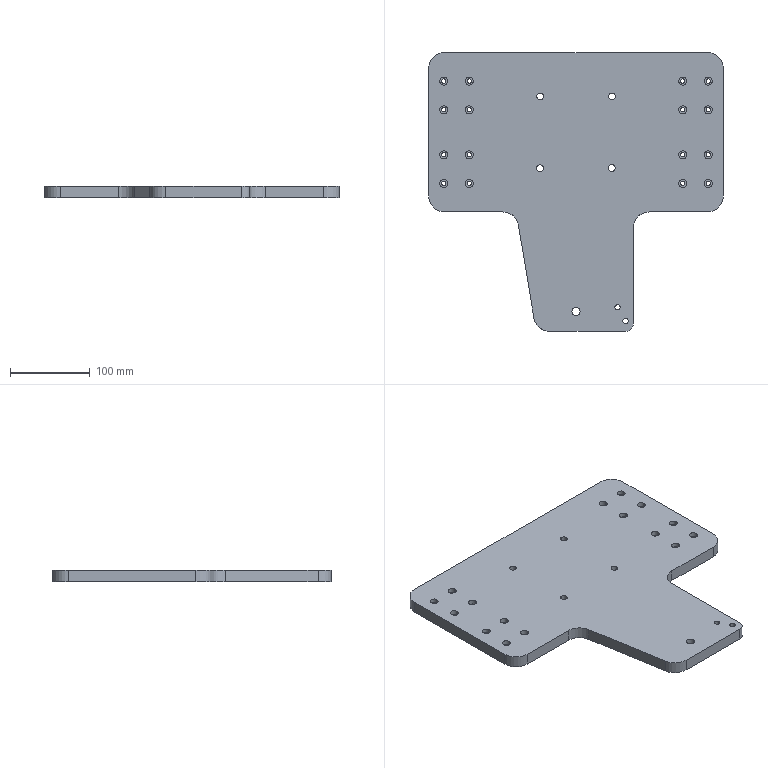Part | SolidWorks | features ICE 4, BaseBody 1, Fillet 1 | 1 solid | 112 faces | box 370 x 350 x 15 mm | volume 1392433 mm3 | cylinder 86 | plane 26 | commonest cylinder face diameters 5.5 x32 10 x32 8.5 x8 40 x7 6.8 x4 10.2 x2